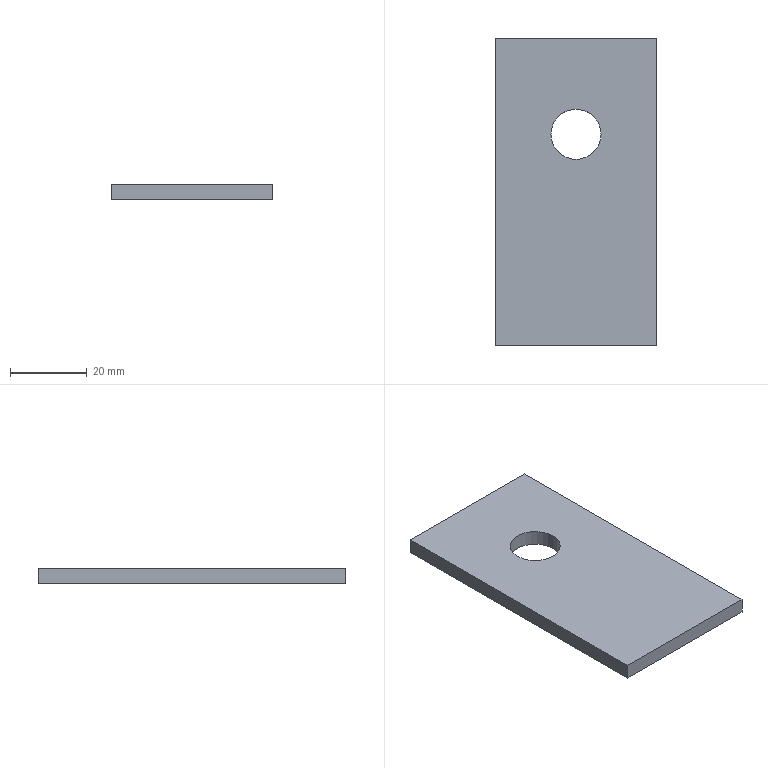Part | SolidWorks | features FlatPattern 1, SMBaseFlange 1, SheetMetal 1 | 1 solid | 8 faces | box 42 x 80 x 4 mm | volume 12909 mm3 | plane 6 | cylinder 2 | commonest cylinder face diameters 13 x2
STEP:
#1=CARTESIAN_POINT('',(-27.5,55.,4.));
#2=VERTEX_POINT('',#1);
#3=CARTESIAN_POINT('',(-14.5,55.,4.));
#4=VERTEX_POINT('',#3);
#5=CARTESIAN_POINT('',(-21.,55.,4.));
#6=DIRECTION('',(0.,0.,1.));
#7=DIRECTION('',(1.,0.,0.));
#8=AXIS2_PLACEMENT_3D('',#5,#6,#7);
#9=CIRCLE('',#8,6.5);
#10=EDGE_CURVE('',#2,#4,#9,.T.);
#11=ORIENTED_EDGE('',*,*,#10,.T.);
#12=CARTESIAN_POINT('',(-14.5,55.,0.));
#13=VERTEX_POINT('',#12);
#14=CARTESIAN_POINT('',(-14.5,55.,4.));
#15=DIRECTION('',(0.,0.,-1.));
#16=VECTOR('',#15,1000.);
#17=LINE('',#14,#16);
#18=EDGE_CURVE('',#4,#13,#17,.T.);
#19=ORIENTED_EDGE('',*,*,#18,.T.);
#20=CARTESIAN_POINT('',(-27.5,55.,0.));
#21=VERTEX_POINT('',#20);
#22=CARTESIAN_POINT('',(-21.,55.,0.));
#23=DIRECTION('',(0.,0.,1.));
#24=DIRECTION('',(1.,0.,0.));
#25=AXIS2_PLACEMENT_3D('',#22,#23,#24);
#26=CIRCLE('',#25,6.5);
#27=EDGE_CURVE('',#21,#13,#26,.T.);
#28=ORIENTED_EDGE('',*,*,#27,.F.);
#29=CARTESIAN_POINT('',(-27.5,55.,4.));
#30=DIRECTION('',(0.,0.,-1.));
#31=VECTOR('',#30,1000.);
#32=LINE('',#29,#31);
#33=EDGE_CURVE('',#2,#21,#32,.T.);
#34=ORIENTED_EDGE('',*,*,#33,.F.);
#35=EDGE_LOOP('',(#11,#19,#28,#34));
#36=FACE_OUTER_BOUND('',#35,.T.);
#37=CARTESIAN_POINT('',(-21.,55.,4.));
#38=DIRECTION('',(0.,0.,-1.));
#39=DIRECTION('',(-1.,0.,0.));
#40=AXIS2_PLACEMENT_3D('',#37,#38,#39);
#41=CYLINDRICAL_SURFACE('',#40,6.5);
#42=ADVANCED_FACE('',(#36),#41,.F.);
#43=CARTESIAN_POINT('',(0.,0.,4.));
#44=VERTEX_POINT('',#43);
#45=CARTESIAN_POINT('',(0.,80.,4.));
#46=VERTEX_POINT('',#45);
#47=CARTESIAN_POINT('',(0.,80.,4.));
#48=DIRECTION('',(0.,1.,0.));
#49=VECTOR('',#48,1000.);
#50=LINE('',#47,#49);
#51=EDGE_CURVE('',#44,#46,#50,.T.);
#52=ORIENTED_EDGE('',*,*,#51,.T.);
#53=CARTESIAN_POINT('',(-42.,80.,4.));
#54=VERTEX_POINT('',#53);
#55=CARTESIAN_POINT('',(-42.,80.,4.));
#56=DIRECTION('',(-1.,0.,0.));
#57=VECTOR('',#56,1000.);
#58=LINE('',#55,#57);
#59=EDGE_CURVE('',#46,#54,#58,.T.);
#60=ORIENTED_EDGE('',*,*,#59,.T.);
#61=CARTESIAN_POINT('',(-42.,0.,4.));
#62=VERTEX_POINT('',#61);
#63=CARTESIAN_POINT('',(-42.,80.,4.));
#64=DIRECTION('',(0.,-1.,0.));
#65=VECTOR('',#64,1000.);
#66=LINE('',#63,#65);
#67=EDGE_CURVE('',#54,#62,#66,.T.);
#68=ORIENTED_EDGE('',*,*,#67,.T.);
#69=CARTESIAN_POINT('',(0.,0.,4.));
#70=DIRECTION('',(1.,0.,0.));
#71=VECTOR('',#70,1000.);
#72=LINE('',#69,#71);
#73=EDGE_CURVE('',#62,#44,#72,.T.);
#74=ORIENTED_EDGE('',*,*,#73,.T.);
#75=EDGE_LOOP('',(#52,#60,#68,#74));
#76=FACE_OUTER_BOUND('',#75,.T.);
#77=ORIENTED_EDGE('',*,*,#10,.F.);
#78=CARTESIAN_POINT('',(-21.,55.,4.));
#79=DIRECTION('',(0.,0.,1.));
#80=DIRECTION('',(1.,0.,0.));
#81=AXIS2_PLACEMENT_3D('',#78,#79,#80);
#82=CIRCLE('',#81,6.5);
#83=EDGE_CURVE('',#4,#2,#82,.T.);
#84=ORIENTED_EDGE('',*,*,#83,.F.);
#85=EDGE_LOOP('',(#77,#84));
#86=FACE_BOUND('',#85,.T.);
#87=CARTESIAN_POINT('',(0.,80.,4.));
#88=DIRECTION('',(0.,0.,1.));
#89=DIRECTION('',(1.,0.,0.));
#90=AXIS2_PLACEMENT_3D('',#87,#88,#89);
#91=PLANE('',#90);
#92=ADVANCED_FACE('',(#76,#86),#91,.T.);
#93=CARTESIAN_POINT('',(0.,0.,0.));
#94=VERTEX_POINT('',#93);
#95=CARTESIAN_POINT('',(0.,80.,0.));
#96=VERTEX_POINT('',#95);
#97=CARTESIAN_POINT('',(0.,80.,0.));
#98=DIRECTION('',(0.,1.,0.));
#99=VECTOR('',#98,1000.);
#100=LINE('',#97,#99);
#101=EDGE_CURVE('',#94,#96,#100,.T.);
#102=ORIENTED_EDGE('',*,*,#101,.F.);
#103=CARTESIAN_POINT('',(-42.,0.,0.));
#104=VERTEX_POINT('',#103);
#105=CARTESIAN_POINT('',(0.,0.,0.));
#106=DIRECTION('',(1.,0.,0.));
#107=VECTOR('',#106,1000.);
#108=LINE('',#105,#107);
#109=EDGE_CURVE('',#104,#94,#108,.T.);
#110=ORIENTED_EDGE('',*,*,#109,.F.);
#111=CARTESIAN_POINT('',(-42.,80.,0.));
#112=VERTEX_POINT('',#111);
#113=CARTESIAN_POINT('',(-42.,80.,0.));
#114=DIRECTION('',(0.,-1.,0.));
#115=VECTOR('',#114,1000.);
#116=LINE('',#113,#115);
#117=EDGE_CURVE('',#112,#104,#116,.T.);
#118=ORIENTED_EDGE('',*,*,#117,.F.);
#119=CARTESIAN_POINT('',(-42.,80.,0.));
#120=DIRECTION('',(-1.,0.,0.));
#121=VECTOR('',#120,1000.);
#122=LINE('',#119,#121);
#123=EDGE_CURVE('',#96,#112,#122,.T.);
#124=ORIENTED_EDGE('',*,*,#123,.F.);
#125=EDGE_LOOP('',(#102,#110,#118,#124));
#126=FACE_OUTER_BOUND('',#125,.T.);
#127=ORIENTED_EDGE('',*,*,#27,.T.);
#128=CARTESIAN_POINT('',(-21.,55.,0.));
#129=DIRECTION('',(0.,0.,1.));
#130=DIRECTION('',(1.,0.,0.));
#131=AXIS2_PLACEMENT_3D('',#128,#129,#130);
#132=CIRCLE('',#131,6.5);
#133=EDGE_CURVE('',#13,#21,#132,.T.);
#134=ORIENTED_EDGE('',*,*,#133,.T.);
#135=EDGE_LOOP('',(#127,#134));
#136=FACE_BOUND('',#135,.T.);
#137=CARTESIAN_POINT('',(0.,80.,0.));
#138=DIRECTION('',(0.,0.,1.));
#139=DIRECTION('',(1.,0.,0.));
#140=AXIS2_PLACEMENT_3D('',#137,#138,#139);
#141=PLANE('',#140);
#142=ADVANCED_FACE('',(#126,#136),#141,.F.);
#143=ORIENTED_EDGE('',*,*,#101,.T.);
#144=CARTESIAN_POINT('',(0.,80.,4.));
#145=DIRECTION('',(0.,0.,-1.));
#146=VECTOR('',#145,1000.);
#147=LINE('',#144,#146);
#148=EDGE_CURVE('',#46,#96,#147,.T.);
#149=ORIENTED_EDGE('',*,*,#148,.F.);
#150=ORIENTED_EDGE('',*,*,#51,.F.);
#151=CARTESIAN_POINT('',(0.,0.,4.));
#152=DIRECTION('',(0.,0.,-1.));
#153=VECTOR('',#152,1000.);
#154=LINE('',#151,#153);
#155=EDGE_CURVE('',#44,#94,#154,.T.);
#156=ORIENTED_EDGE('',*,*,#155,.T.);
#157=EDGE_LOOP('',(#143,#149,#150,#156));
#158=FACE_OUTER_BOUND('',#157,.T.);
#159=CARTESIAN_POINT('',(0.,80.,4.));
#160=DIRECTION('',(-1.,0.,0.));
#161=DIRECTION('',(0.,-1.,0.));
#162=AXIS2_PLACEMENT_3D('',#159,#160,#161);
#163=PLANE('',#162);
#164=ADVANCED_FACE('',(#158),#163,.F.);
#165=ORIENTED_EDGE('',*,*,#123,.T.);
#166=CARTESIAN_POINT('',(-42.,80.,4.));
#167=DIRECTION('',(0.,0.,-1.));
#168=VECTOR('',#167,1000.);
#169=LINE('',#166,#168);
#170=EDGE_CURVE('',#54,#112,#169,.T.);
#171=ORIENTED_EDGE('',*,*,#170,.F.);
#172=ORIENTED_EDGE('',*,*,#59,.F.);
#173=ORIENTED_EDGE('',*,*,#148,.T.);
#174=EDGE_LOOP('',(#165,#171,#172,#173));
#175=FACE_OUTER_BOUND('',#174,.T.);
#176=CARTESIAN_POINT('',(-42.,80.,4.));
#177=DIRECTION('',(0.,-1.,0.));
#178=DIRECTION('',(0.,0.,-1.));
#179=AXIS2_PLACEMENT_3D('',#176,#177,#178);
#180=PLANE('',#179);
#181=ADVANCED_FACE('',(#175),#180,.F.);
#182=ORIENTED_EDGE('',*,*,#117,.T.);
#183=CARTESIAN_POINT('',(-42.,0.,4.));
#184=DIRECTION('',(0.,0.,-1.));
#185=VECTOR('',#184,1000.);
#186=LINE('',#183,#185);
#187=EDGE_CURVE('',#62,#104,#186,.T.);
#188=ORIENTED_EDGE('',*,*,#187,.F.);
#189=ORIENTED_EDGE('',*,*,#67,.F.);
#190=ORIENTED_EDGE('',*,*,#170,.T.);
#191=EDGE_LOOP('',(#182,#188,#189,#190));
#192=FACE_OUTER_BOUND('',#191,.T.);
#193=CARTESIAN_POINT('',(-42.,80.,4.));
#194=DIRECTION('',(1.,0.,0.));
#195=DIRECTION('',(0.,1.,0.));
#196=AXIS2_PLACEMENT_3D('',#193,#194,#195);
#197=PLANE('',#196);
#198=ADVANCED_FACE('',(#192),#197,.F.);
#199=ORIENTED_EDGE('',*,*,#109,.T.);
#200=ORIENTED_EDGE('',*,*,#155,.F.);
#201=ORIENTED_EDGE('',*,*,#73,.F.);
#202=ORIENTED_EDGE('',*,*,#187,.T.);
#203=EDGE_LOOP('',(#199,#200,#201,#202));
#204=FACE_OUTER_BOUND('',#203,.T.);
#205=CARTESIAN_POINT('',(0.,0.,4.));
#206=DIRECTION('',(0.,1.,0.));
#207=DIRECTION('',(-1.,0.,0.));
#208=AXIS2_PLACEMENT_3D('',#205,#206,#207);
#209=PLANE('',#208);
#210=ADVANCED_FACE('',(#204),#209,.F.);
#211=ORIENTED_EDGE('',*,*,#18,.F.);
#212=ORIENTED_EDGE('',*,*,#83,.T.);
#213=ORIENTED_EDGE('',*,*,#33,.T.);
#214=ORIENTED_EDGE('',*,*,#133,.F.);
#215=EDGE_LOOP('',(#211,#212,#213,#214));
#216=FACE_OUTER_BOUND('',#215,.T.);
#217=CARTESIAN_POINT('',(-21.,55.,4.));
#218=DIRECTION('',(0.,0.,-1.));
#219=DIRECTION('',(-1.,0.,0.));
#220=AXIS2_PLACEMENT_3D('',#217,#218,#219);
#221=CYLINDRICAL_SURFACE('',#220,6.5);
#222=ADVANCED_FACE('',(#216),#221,.F.);
#223=CLOSED_SHELL('',(#42,#92,#142,#164,#181,#198,#210,#222));
#224=MANIFOLD_SOLID_BREP('',#223);
#225=CARTESIAN_POINT('',(0.,0.,0.));
#226=DIRECTION('',(0.,0.,1.));
#227=DIRECTION('',(1.,0.,0.));
#228=AXIS2_PLACEMENT_3D('',#225,#226,#227);
#229=(LENGTH_UNIT()NAMED_UNIT(*)SI_UNIT(.MILLI.,.METRE.));
#230=UNCERTAINTY_MEASURE_WITH_UNIT(LENGTH_MEASURE(0.00001),#229,'','');
#231=(NAMED_UNIT(*)PLANE_ANGLE_UNIT()SI_UNIT($,.RADIAN.));
#232=(NAMED_UNIT(*)SI_UNIT($,.STERADIAN.)SOLID_ANGLE_UNIT());
#233=(GEOMETRIC_REPRESENTATION_CONTEXT(3)GLOBAL_UNCERTAINTY_ASSIGNED_CONTEXT((#230))GLOBAL_UNIT_ASSIGNED_CONTEXT((#229,#231,#232))REPRESENTATION_CONTEXT('',''));
#234=ADVANCED_BREP_SHAPE_REPRESENTATION('',(#224,#228),#233);